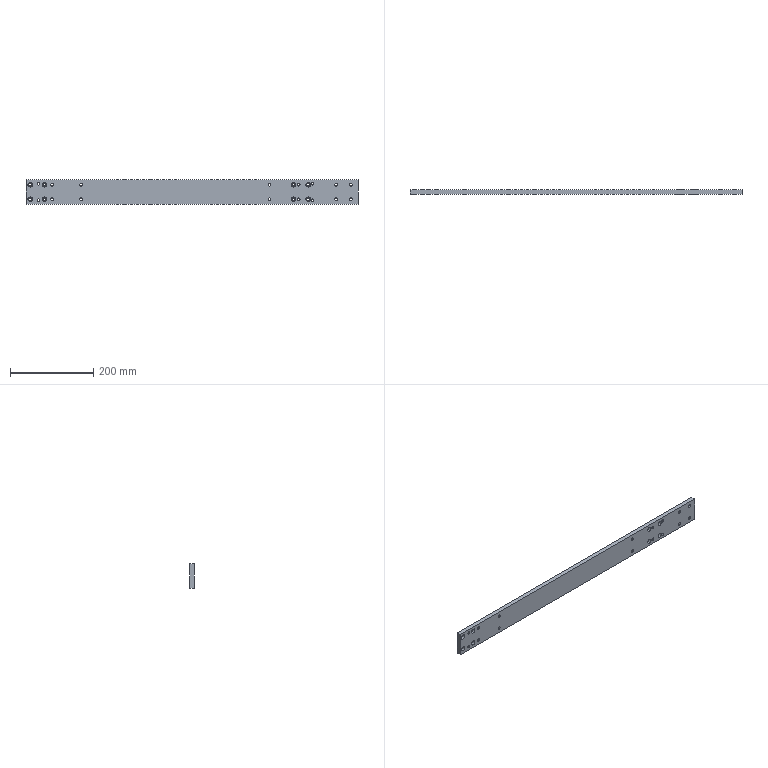Part | STEP file | 打磨单元二底Plate | 1 solid | 78 faces | box 800 x 10 x 60 mm | volume 468480 mm3 | cylinder 64 | plane 14 | commonest cylinder face diameters 6.6 x48 11 x16